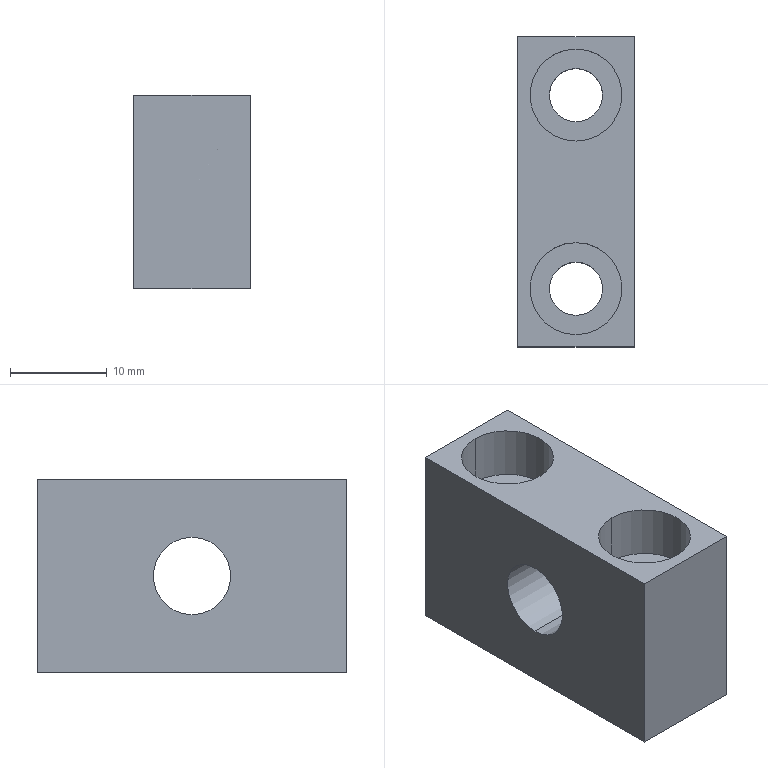Part | STEP file | TNSN20-Y20-F22-Part-13 | 1 solid | 18 faces | box 12 x 32 x 20 mm | volume 5608 mm3 | cylinder 10 | plane 8 | commonest cylinder face diameters 5.5 x4 9.5 x4 8 x2
STEP:
#1=CARTESIAN_POINT('',(14045.745,13720.046,23.));
#2=VERTEX_POINT('',#1);
#3=CARTESIAN_POINT('',(14045.745,13720.046,15.));
#4=VERTEX_POINT('',#3);
#5=CARTESIAN_POINT('',(14045.745,13720.046,19.));
#6=DIRECTION('',(1.,0.,0.));
#7=DIRECTION('',(0.,1.,0.));
#8=AXIS2_PLACEMENT_3D('',#5,#6,#7);
#9=CIRCLE('',#8,4.);
#10=EDGE_CURVE('',#2,#4,#9,.T.);
#11=ORIENTED_EDGE('',*,*,#10,.T.);
#12=CARTESIAN_POINT('',(14033.745,13720.046,15.));
#13=VERTEX_POINT('',#12);
#14=CARTESIAN_POINT('',(14045.745,13720.046,15.));
#15=DIRECTION('',(-1.,0.,0.));
#16=VECTOR('',#15,1000.);
#17=LINE('',#14,#16);
#18=EDGE_CURVE('',#4,#13,#17,.T.);
#19=ORIENTED_EDGE('',*,*,#18,.T.);
#20=CARTESIAN_POINT('',(14033.745,13720.046,23.));
#21=VERTEX_POINT('',#20);
#22=CARTESIAN_POINT('',(14033.745,13720.046,19.));
#23=DIRECTION('',(1.,0.,0.));
#24=DIRECTION('',(0.,1.,0.));
#25=AXIS2_PLACEMENT_3D('',#22,#23,#24);
#26=CIRCLE('',#25,4.);
#27=EDGE_CURVE('',#21,#13,#26,.T.);
#28=ORIENTED_EDGE('',*,*,#27,.F.);
#29=CARTESIAN_POINT('',(14045.745,13720.046,23.));
#30=DIRECTION('',(-1.,0.,0.));
#31=VECTOR('',#30,1000.);
#32=LINE('',#29,#31);
#33=EDGE_CURVE('',#2,#21,#32,.T.);
#34=ORIENTED_EDGE('',*,*,#33,.F.);
#35=EDGE_LOOP('',(#11,#19,#28,#34));
#36=FACE_OUTER_BOUND('',#35,.T.);
#37=CARTESIAN_POINT('',(14045.745,13720.046,19.));
#38=DIRECTION('',(-1.,0.,0.));
#39=DIRECTION('',(0.,0.,1.));
#40=AXIS2_PLACEMENT_3D('',#37,#38,#39);
#41=CYLINDRICAL_SURFACE('',#40,4.);
#42=ADVANCED_FACE('',(#36),#41,.F.);
#43=CARTESIAN_POINT('',(14039.745,13714.796,23.5));
#44=VERTEX_POINT('',#43);
#45=CARTESIAN_POINT('',(14039.745,13705.296,23.5));
#46=VERTEX_POINT('',#45);
#47=CARTESIAN_POINT('',(14039.745,13710.046,23.5));
#48=DIRECTION('',(0.,0.,1.));
#49=DIRECTION('',(1.,0.,0.));
#50=AXIS2_PLACEMENT_3D('',#47,#48,#49);
#51=CIRCLE('',#50,4.75);
#52=EDGE_CURVE('',#44,#46,#51,.T.);
#53=ORIENTED_EDGE('',*,*,#52,.F.);
#54=CARTESIAN_POINT('',(14039.745,13714.796,29.));
#55=VERTEX_POINT('',#54);
#56=CARTESIAN_POINT('',(14039.745,13714.796,26.25));
#57=DIRECTION('',(0.,0.,1.));
#58=VECTOR('',#57,1000.);
#59=LINE('',#56,#58);
#60=EDGE_CURVE('',#44,#55,#59,.T.);
#61=ORIENTED_EDGE('',*,*,#60,.T.);
#62=CARTESIAN_POINT('',(14039.745,13705.296,29.));
#63=VERTEX_POINT('',#62);
#64=CARTESIAN_POINT('',(14039.745,13710.046,29.));
#65=DIRECTION('',(0.,0.,1.));
#66=DIRECTION('',(1.,0.,0.));
#67=AXIS2_PLACEMENT_3D('',#64,#65,#66);
#68=CIRCLE('',#67,4.75);
#69=EDGE_CURVE('',#55,#63,#68,.T.);
#70=ORIENTED_EDGE('',*,*,#69,.T.);
#71=CARTESIAN_POINT('',(14039.745,13705.296,26.25));
#72=DIRECTION('',(0.,0.,1.));
#73=VECTOR('',#72,1000.);
#74=LINE('',#71,#73);
#75=EDGE_CURVE('',#46,#63,#74,.T.);
#76=ORIENTED_EDGE('',*,*,#75,.F.);
#77=EDGE_LOOP('',(#53,#61,#70,#76));
#78=FACE_OUTER_BOUND('',#77,.T.);
#79=CARTESIAN_POINT('',(14039.745,13710.046,26.25));
#80=DIRECTION('',(0.,0.,1.));
#81=DIRECTION('',(0.,-1.,0.));
#82=AXIS2_PLACEMENT_3D('',#79,#80,#81);
#83=CYLINDRICAL_SURFACE('',#82,4.75);
#84=ADVANCED_FACE('',(#78),#83,.F.);
#85=CARTESIAN_POINT('',(14039.745,13734.796,23.5));
#86=VERTEX_POINT('',#85);
#87=CARTESIAN_POINT('',(14039.745,13725.296,23.5));
#88=VERTEX_POINT('',#87);
#89=CARTESIAN_POINT('',(14039.745,13730.046,23.5));
#90=DIRECTION('',(0.,0.,1.));
#91=DIRECTION('',(1.,0.,0.));
#92=AXIS2_PLACEMENT_3D('',#89,#90,#91);
#93=CIRCLE('',#92,4.75);
#94=EDGE_CURVE('',#86,#88,#93,.T.);
#95=ORIENTED_EDGE('',*,*,#94,.F.);
#96=CARTESIAN_POINT('',(14039.745,13734.796,29.));
#97=VERTEX_POINT('',#96);
#98=CARTESIAN_POINT('',(14039.745,13734.796,26.25));
#99=DIRECTION('',(0.,0.,1.));
#100=VECTOR('',#99,1000.);
#101=LINE('',#98,#100);
#102=EDGE_CURVE('',#86,#97,#101,.T.);
#103=ORIENTED_EDGE('',*,*,#102,.T.);
#104=CARTESIAN_POINT('',(14039.745,13725.296,29.));
#105=VERTEX_POINT('',#104);
#106=CARTESIAN_POINT('',(14039.745,13730.046,29.));
#107=DIRECTION('',(0.,0.,1.));
#108=DIRECTION('',(1.,0.,0.));
#109=AXIS2_PLACEMENT_3D('',#106,#107,#108);
#110=CIRCLE('',#109,4.75);
#111=EDGE_CURVE('',#97,#105,#110,.T.);
#112=ORIENTED_EDGE('',*,*,#111,.T.);
#113=CARTESIAN_POINT('',(14039.745,13725.296,26.25));
#114=DIRECTION('',(0.,0.,1.));
#115=VECTOR('',#114,1000.);
#116=LINE('',#113,#115);
#117=EDGE_CURVE('',#88,#105,#116,.T.);
#118=ORIENTED_EDGE('',*,*,#117,.F.);
#119=EDGE_LOOP('',(#95,#103,#112,#118));
#120=FACE_OUTER_BOUND('',#119,.T.);
#121=CARTESIAN_POINT('',(14039.745,13730.046,26.25));
#122=DIRECTION('',(0.,0.,1.));
#123=DIRECTION('',(0.,-1.,0.));
#124=AXIS2_PLACEMENT_3D('',#121,#122,#123);
#125=CYLINDRICAL_SURFACE('',#124,4.75);
#126=ADVANCED_FACE('',(#120),#125,.F.);
#127=CARTESIAN_POINT('',(14039.745,13707.296,23.5));
#128=VERTEX_POINT('',#127);
#129=CARTESIAN_POINT('',(14039.745,13712.796,23.5));
#130=VERTEX_POINT('',#129);
#131=CARTESIAN_POINT('',(14039.745,13710.046,23.5));
#132=DIRECTION('',(0.,0.,1.));
#133=DIRECTION('',(0.,-1.,0.));
#134=AXIS2_PLACEMENT_3D('',#131,#132,#133);
#135=CIRCLE('',#134,2.75);
#136=EDGE_CURVE('',#128,#130,#135,.T.);
#137=ORIENTED_EDGE('',*,*,#136,.T.);
#138=CARTESIAN_POINT('',(14039.745,13712.796,9.));
#139=VERTEX_POINT('',#138);
#140=CARTESIAN_POINT('',(14039.745,13712.796,16.25));
#141=DIRECTION('',(0.,0.,-1.));
#142=VECTOR('',#141,1000.);
#143=LINE('',#140,#142);
#144=EDGE_CURVE('',#130,#139,#143,.T.);
#145=ORIENTED_EDGE('',*,*,#144,.T.);
#146=CARTESIAN_POINT('',(14039.745,13707.296,9.));
#147=VERTEX_POINT('',#146);
#148=CARTESIAN_POINT('',(14039.745,13710.046,9.));
#149=DIRECTION('',(0.,0.,-1.));
#150=DIRECTION('',(0.,1.,0.));
#151=AXIS2_PLACEMENT_3D('',#148,#149,#150);
#152=CIRCLE('',#151,2.75);
#153=EDGE_CURVE('',#139,#147,#152,.T.);
#154=ORIENTED_EDGE('',*,*,#153,.T.);
#155=CARTESIAN_POINT('',(14039.745,13707.296,16.25));
#156=DIRECTION('',(0.,0.,-1.));
#157=VECTOR('',#156,1000.);
#158=LINE('',#155,#157);
#159=EDGE_CURVE('',#128,#147,#158,.T.);
#160=ORIENTED_EDGE('',*,*,#159,.F.);
#161=EDGE_LOOP('',(#137,#145,#154,#160));
#162=FACE_OUTER_BOUND('',#161,.T.);
#163=CARTESIAN_POINT('',(14039.745,13710.046,16.25));
#164=DIRECTION('',(0.,0.,-1.));
#165=DIRECTION('',(0.,-1.,0.));
#166=AXIS2_PLACEMENT_3D('',#163,#164,#165);
#167=CYLINDRICAL_SURFACE('',#166,2.75);
#168=ADVANCED_FACE('',(#162),#167,.F.);
#169=CARTESIAN_POINT('',(14039.745,13727.296,23.5));
#170=VERTEX_POINT('',#169);
#171=CARTESIAN_POINT('',(14039.745,13732.796,23.5));
#172=VERTEX_POINT('',#171);
#173=CARTESIAN_POINT('',(14039.745,13730.046,23.5));
#174=DIRECTION('',(0.,0.,1.));
#175=DIRECTION('',(0.,-1.,0.));
#176=AXIS2_PLACEMENT_3D('',#173,#174,#175);
#177=CIRCLE('',#176,2.75);
#178=EDGE_CURVE('',#170,#172,#177,.T.);
#179=ORIENTED_EDGE('',*,*,#178,.T.);
#180=CARTESIAN_POINT('',(14039.745,13732.796,9.));
#181=VERTEX_POINT('',#180);
#182=CARTESIAN_POINT('',(14039.745,13732.796,16.25));
#183=DIRECTION('',(0.,0.,-1.));
#184=VECTOR('',#183,1000.);
#185=LINE('',#182,#184);
#186=EDGE_CURVE('',#172,#181,#185,.T.);
#187=ORIENTED_EDGE('',*,*,#186,.T.);
#188=CARTESIAN_POINT('',(14039.745,13727.296,9.));
#189=VERTEX_POINT('',#188);
#190=CARTESIAN_POINT('',(14039.745,13730.046,9.));
#191=DIRECTION('',(0.,0.,-1.));
#192=DIRECTION('',(0.,1.,0.));
#193=AXIS2_PLACEMENT_3D('',#190,#191,#192);
#194=CIRCLE('',#193,2.75);
#195=EDGE_CURVE('',#181,#189,#194,.T.);
#196=ORIENTED_EDGE('',*,*,#195,.T.);
#197=CARTESIAN_POINT('',(14039.745,13727.296,16.25));
#198=DIRECTION('',(0.,0.,-1.));
#199=VECTOR('',#198,1000.);
#200=LINE('',#197,#199);
#201=EDGE_CURVE('',#170,#189,#200,.T.);
#202=ORIENTED_EDGE('',*,*,#201,.F.);
#203=EDGE_LOOP('',(#179,#187,#196,#202));
#204=FACE_OUTER_BOUND('',#203,.T.);
#205=CARTESIAN_POINT('',(14039.745,13730.046,16.25));
#206=DIRECTION('',(0.,0.,-1.));
#207=DIRECTION('',(0.,-1.,0.));
#208=AXIS2_PLACEMENT_3D('',#205,#206,#207);
#209=CYLINDRICAL_SURFACE('',#208,2.75);
#210=ADVANCED_FACE('',(#204),#209,.F.);
#211=CARTESIAN_POINT('',(14045.745,13736.046,29.));
#212=VERTEX_POINT('',#211);
#213=CARTESIAN_POINT('',(14033.745,13736.046,29.));
#214=VERTEX_POINT('',#213);
#215=CARTESIAN_POINT('',(14045.745,13736.046,29.));
#216=DIRECTION('',(-1.,0.,0.));
#217=VECTOR('',#216,1000.);
#218=LINE('',#215,#217);
#219=EDGE_CURVE('',#212,#214,#218,.T.);
#220=ORIENTED_EDGE('',*,*,#219,.T.);
#221=CARTESIAN_POINT('',(14033.745,13704.046,29.));
#222=VERTEX_POINT('',#221);
#223=CARTESIAN_POINT('',(14033.745,13704.046,29.));
#224=DIRECTION('',(0.,1.,0.));
#225=VECTOR('',#224,1000.);
#226=LINE('',#223,#225);
#227=EDGE_CURVE('',#222,#214,#226,.T.);
#228=ORIENTED_EDGE('',*,*,#227,.F.);
#229=CARTESIAN_POINT('',(14045.745,13704.046,29.));
#230=VERTEX_POINT('',#229);
#231=CARTESIAN_POINT('',(14045.745,13704.046,29.));
#232=DIRECTION('',(-1.,0.,0.));
#233=VECTOR('',#232,1000.);
#234=LINE('',#231,#233);
#235=EDGE_CURVE('',#230,#222,#234,.T.);
#236=ORIENTED_EDGE('',*,*,#235,.F.);
#237=CARTESIAN_POINT('',(14045.745,13704.046,29.));
#238=DIRECTION('',(0.,1.,0.));
#239=VECTOR('',#238,1000.);
#240=LINE('',#237,#239);
#241=EDGE_CURVE('',#230,#212,#240,.T.);
#242=ORIENTED_EDGE('',*,*,#241,.T.);
#243=EDGE_LOOP('',(#220,#228,#236,#242));
#244=FACE_OUTER_BOUND('',#243,.T.);
#245=CARTESIAN_POINT('',(14039.745,13710.046,29.));
#246=DIRECTION('',(0.,0.,1.));
#247=DIRECTION('',(1.,0.,0.));
#248=AXIS2_PLACEMENT_3D('',#245,#246,#247);
#249=CIRCLE('',#248,4.75);
#250=EDGE_CURVE('',#63,#55,#249,.T.);
#251=ORIENTED_EDGE('',*,*,#250,.F.);
#252=ORIENTED_EDGE('',*,*,#69,.F.);
#253=EDGE_LOOP('',(#251,#252));
#254=FACE_BOUND('',#253,.T.);
#255=CARTESIAN_POINT('',(14039.745,13730.046,29.));
#256=DIRECTION('',(0.,0.,1.));
#257=DIRECTION('',(1.,0.,0.));
#258=AXIS2_PLACEMENT_3D('',#255,#256,#257);
#259=CIRCLE('',#258,4.75);
#260=EDGE_CURVE('',#105,#97,#259,.T.);
#261=ORIENTED_EDGE('',*,*,#260,.F.);
#262=ORIENTED_EDGE('',*,*,#111,.F.);
#263=EDGE_LOOP('',(#261,#262));
#264=FACE_BOUND('',#263,.T.);
#265=CARTESIAN_POINT('',(14008.285,13690.337,29.));
#266=DIRECTION('',(0.,0.,-1.));
#267=DIRECTION('',(0.,1.,0.));
#268=AXIS2_PLACEMENT_3D('',#265,#266,#267);
#269=PLANE('',#268);
#270=ADVANCED_FACE('',(#244,#254,#264),#269,.F.);
#271=CARTESIAN_POINT('',(14033.745,13736.046,9.));
#272=VERTEX_POINT('',#271);
#273=CARTESIAN_POINT('',(14033.745,13736.046,29.));
#274=DIRECTION('',(0.,0.,-1.));
#275=VECTOR('',#274,1000.);
#276=LINE('',#273,#275);
#277=EDGE_CURVE('',#214,#272,#276,.T.);
#278=ORIENTED_EDGE('',*,*,#277,.T.);
#279=CARTESIAN_POINT('',(14033.745,13704.046,9.));
#280=VERTEX_POINT('',#279);
#281=CARTESIAN_POINT('',(14033.745,13704.046,9.));
#282=DIRECTION('',(0.,1.,0.));
#283=VECTOR('',#282,1000.);
#284=LINE('',#281,#283);
#285=EDGE_CURVE('',#280,#272,#284,.T.);
#286=ORIENTED_EDGE('',*,*,#285,.F.);
#287=CARTESIAN_POINT('',(14033.745,13704.046,29.));
#288=DIRECTION('',(0.,0.,-1.));
#289=VECTOR('',#288,1000.);
#290=LINE('',#287,#289);
#291=EDGE_CURVE('',#222,#280,#290,.T.);
#292=ORIENTED_EDGE('',*,*,#291,.F.);
#293=ORIENTED_EDGE('',*,*,#227,.T.);
#294=EDGE_LOOP('',(#278,#286,#292,#293));
#295=FACE_OUTER_BOUND('',#294,.T.);
#296=ORIENTED_EDGE('',*,*,#27,.T.);
#297=CARTESIAN_POINT('',(14033.745,13720.046,19.));
#298=DIRECTION('',(1.,0.,0.));
#299=DIRECTION('',(0.,1.,0.));
#300=AXIS2_PLACEMENT_3D('',#297,#298,#299);
#301=CIRCLE('',#300,4.);
#302=EDGE_CURVE('',#13,#21,#301,.T.);
#303=ORIENTED_EDGE('',*,*,#302,.T.);
#304=EDGE_LOOP('',(#296,#303));
#305=FACE_BOUND('',#304,.T.);
#306=CARTESIAN_POINT('',(14033.745,13691.744,-9.302));
#307=DIRECTION('',(1.,0.,0.));
#308=DIRECTION('',(0.,1.,0.));
#309=AXIS2_PLACEMENT_3D('',#306,#307,#308);
#310=PLANE('',#309);
#311=ADVANCED_FACE('',(#295,#305),#310,.F.);
#312=CARTESIAN_POINT('',(14045.745,13736.046,9.));
#313=VERTEX_POINT('',#312);
#314=CARTESIAN_POINT('',(14033.745,13736.046,9.));
#315=DIRECTION('',(1.,0.,0.));
#316=VECTOR('',#315,1000.);
#317=LINE('',#314,#316);
#318=EDGE_CURVE('',#272,#313,#317,.T.);
#319=ORIENTED_EDGE('',*,*,#318,.T.);
#320=CARTESIAN_POINT('',(14045.745,13704.046,9.));
#321=VERTEX_POINT('',#320);
#322=CARTESIAN_POINT('',(14045.745,13704.046,9.));
#323=DIRECTION('',(0.,1.,0.));
#324=VECTOR('',#323,1000.);
#325=LINE('',#322,#324);
#326=EDGE_CURVE('',#321,#313,#325,.T.);
#327=ORIENTED_EDGE('',*,*,#326,.F.);
#328=CARTESIAN_POINT('',(14033.745,13704.046,9.));
#329=DIRECTION('',(1.,0.,0.));
#330=VECTOR('',#329,1000.);
#331=LINE('',#328,#330);
#332=EDGE_CURVE('',#280,#321,#331,.T.);
#333=ORIENTED_EDGE('',*,*,#332,.F.);
#334=ORIENTED_EDGE('',*,*,#285,.T.);
#335=EDGE_LOOP('',(#319,#327,#333,#334));
#336=FACE_OUTER_BOUND('',#335,.T.);
#337=CARTESIAN_POINT('',(14039.745,13710.046,9.));
#338=DIRECTION('',(0.,0.,-1.));
#339=DIRECTION('',(0.,1.,0.));
#340=AXIS2_PLACEMENT_3D('',#337,#338,#339);
#341=CIRCLE('',#340,2.75);
#342=EDGE_CURVE('',#147,#139,#341,.T.);
#343=ORIENTED_EDGE('',*,*,#342,.F.);
#344=ORIENTED_EDGE('',*,*,#153,.F.);
#345=EDGE_LOOP('',(#343,#344));
#346=FACE_BOUND('',#345,.T.);
#347=CARTESIAN_POINT('',(14039.745,13730.046,9.));
#348=DIRECTION('',(0.,0.,-1.));
#349=DIRECTION('',(0.,1.,0.));
#350=AXIS2_PLACEMENT_3D('',#347,#348,#349);
#351=CIRCLE('',#350,2.75);
#352=EDGE_CURVE('',#189,#181,#351,.T.);
#353=ORIENTED_EDGE('',*,*,#352,.F.);
#354=ORIENTED_EDGE('',*,*,#195,.F.);
#355=EDGE_LOOP('',(#353,#354));
#356=FACE_BOUND('',#355,.T.);
#357=CARTESIAN_POINT('',(14014.113,13745.678,9.));
#358=DIRECTION('',(0.,0.,1.));
#359=DIRECTION('',(0.,-1.,0.));
#360=AXIS2_PLACEMENT_3D('',#357,#358,#359);
#361=PLANE('',#360);
#362=ADVANCED_FACE('',(#336,#346,#356),#361,.F.);
#363=CARTESIAN_POINT('',(14045.745,13736.046,9.));
#364=DIRECTION('',(0.,0.,1.));
#365=VECTOR('',#364,1000.);
#366=LINE('',#363,#365);
#367=EDGE_CURVE('',#313,#212,#366,.T.);
#368=ORIENTED_EDGE('',*,*,#367,.T.);
#369=ORIENTED_EDGE('',*,*,#241,.F.);
#370=CARTESIAN_POINT('',(14045.745,13704.046,9.));
#371=DIRECTION('',(0.,0.,1.));
#372=VECTOR('',#371,1000.);
#373=LINE('',#370,#372);
#374=EDGE_CURVE('',#321,#230,#373,.T.);
#375=ORIENTED_EDGE('',*,*,#374,.F.);
#376=ORIENTED_EDGE('',*,*,#326,.T.);
#377=EDGE_LOOP('',(#368,#369,#375,#376));
#378=FACE_OUTER_BOUND('',#377,.T.);
#379=ORIENTED_EDGE('',*,*,#10,.F.);
#380=CARTESIAN_POINT('',(14045.745,13720.046,19.));
#381=DIRECTION('',(1.,0.,0.));
#382=DIRECTION('',(0.,1.,0.));
#383=AXIS2_PLACEMENT_3D('',#380,#381,#382);
#384=CIRCLE('',#383,4.);
#385=EDGE_CURVE('',#4,#2,#384,.T.);
#386=ORIENTED_EDGE('',*,*,#385,.F.);
#387=EDGE_LOOP('',(#379,#386));
#388=FACE_BOUND('',#387,.T.);
#389=CARTESIAN_POINT('',(14045.745,13748.348,-9.302));
#390=DIRECTION('',(-1.,0.,0.));
#391=DIRECTION('',(0.,-1.,0.));
#392=AXIS2_PLACEMENT_3D('',#389,#390,#391);
#393=PLANE('',#392);
#394=ADVANCED_FACE('',(#378,#388),#393,.F.);
#395=ORIENTED_EDGE('',*,*,#235,.T.);
#396=ORIENTED_EDGE('',*,*,#291,.T.);
#397=ORIENTED_EDGE('',*,*,#332,.T.);
#398=ORIENTED_EDGE('',*,*,#374,.T.);
#399=EDGE_LOOP('',(#395,#396,#397,#398));
#400=FACE_OUTER_BOUND('',#399,.T.);
#401=CARTESIAN_POINT('',(14022.252,13704.046,1.507));
#402=DIRECTION('',(0.,-1.,0.));
#403=DIRECTION('',(1.,0.,0.));
#404=AXIS2_PLACEMENT_3D('',#401,#402,#403);
#405=PLANE('',#404);
#406=ADVANCED_FACE('',(#400),#405,.T.);
#407=ORIENTED_EDGE('',*,*,#219,.F.);
#408=ORIENTED_EDGE('',*,*,#367,.F.);
#409=ORIENTED_EDGE('',*,*,#318,.F.);
#410=ORIENTED_EDGE('',*,*,#277,.F.);
#411=EDGE_LOOP('',(#407,#408,#409,#410));
#412=FACE_OUTER_BOUND('',#411,.T.);
#413=CARTESIAN_POINT('',(14022.252,13736.046,1.507));
#414=DIRECTION('',(0.,-1.,0.));
#415=DIRECTION('',(1.,0.,0.));
#416=AXIS2_PLACEMENT_3D('',#413,#414,#415);
#417=PLANE('',#416);
#418=ADVANCED_FACE('',(#412),#417,.F.);
#419=CARTESIAN_POINT('',(14039.745,13730.046,23.5));
#420=DIRECTION('',(0.,0.,1.));
#421=DIRECTION('',(1.,0.,0.));
#422=AXIS2_PLACEMENT_3D('',#419,#420,#421);
#423=CIRCLE('',#422,4.75);
#424=EDGE_CURVE('',#88,#86,#423,.T.);
#425=ORIENTED_EDGE('',*,*,#424,.T.);
#426=ORIENTED_EDGE('',*,*,#94,.T.);
#427=EDGE_LOOP('',(#425,#426));
#428=FACE_OUTER_BOUND('',#427,.T.);
#429=ORIENTED_EDGE('',*,*,#178,.F.);
#430=CARTESIAN_POINT('',(14039.745,13730.046,23.5));
#431=DIRECTION('',(0.,0.,1.));
#432=DIRECTION('',(0.,-1.,0.));
#433=AXIS2_PLACEMENT_3D('',#430,#431,#432);
#434=CIRCLE('',#433,2.75);
#435=EDGE_CURVE('',#172,#170,#434,.T.);
#436=ORIENTED_EDGE('',*,*,#435,.F.);
#437=EDGE_LOOP('',(#429,#436));
#438=FACE_BOUND('',#437,.T.);
#439=CARTESIAN_POINT('',(14021.045,13746.378,23.5));
#440=DIRECTION('',(0.,0.,1.));
#441=DIRECTION('',(0.,-1.,0.));
#442=AXIS2_PLACEMENT_3D('',#439,#440,#441);
#443=PLANE('',#442);
#444=ADVANCED_FACE('',(#428,#438),#443,.T.);
#445=CARTESIAN_POINT('',(14039.745,13710.046,23.5));
#446=DIRECTION('',(0.,0.,1.));
#447=DIRECTION('',(1.,0.,0.));
#448=AXIS2_PLACEMENT_3D('',#445,#446,#447);
#449=CIRCLE('',#448,4.75);
#450=EDGE_CURVE('',#46,#44,#449,.T.);
#451=ORIENTED_EDGE('',*,*,#450,.T.);
#452=ORIENTED_EDGE('',*,*,#52,.T.);
#453=EDGE_LOOP('',(#451,#452));
#454=FACE_OUTER_BOUND('',#453,.T.);
#455=ORIENTED_EDGE('',*,*,#136,.F.);
#456=CARTESIAN_POINT('',(14039.745,13710.046,23.5));
#457=DIRECTION('',(0.,0.,1.));
#458=DIRECTION('',(0.,-1.,0.));
#459=AXIS2_PLACEMENT_3D('',#456,#457,#458);
#460=CIRCLE('',#459,2.75);
#461=EDGE_CURVE('',#130,#128,#460,.T.);
#462=ORIENTED_EDGE('',*,*,#461,.F.);
#463=EDGE_LOOP('',(#455,#462));
#464=FACE_BOUND('',#463,.T.);
#465=CARTESIAN_POINT('',(14021.045,13726.378,23.5));
#466=DIRECTION('',(0.,0.,1.));
#467=DIRECTION('',(0.,-1.,0.));
#468=AXIS2_PLACEMENT_3D('',#465,#466,#467);
#469=PLANE('',#468);
#470=ADVANCED_FACE('',(#454,#464),#469,.T.);
#471=ORIENTED_EDGE('',*,*,#186,.F.);
#472=ORIENTED_EDGE('',*,*,#435,.T.);
#473=ORIENTED_EDGE('',*,*,#201,.T.);
#474=ORIENTED_EDGE('',*,*,#352,.T.);
#475=EDGE_LOOP('',(#471,#472,#473,#474));
#476=FACE_OUTER_BOUND('',#475,.T.);
#477=CARTESIAN_POINT('',(14039.745,13730.046,16.25));
#478=DIRECTION('',(0.,0.,-1.));
#479=DIRECTION('',(0.,-1.,0.));
#480=AXIS2_PLACEMENT_3D('',#477,#478,#479);
#481=CYLINDRICAL_SURFACE('',#480,2.75);
#482=ADVANCED_FACE('',(#476),#481,.F.);
#483=ORIENTED_EDGE('',*,*,#144,.F.);
#484=ORIENTED_EDGE('',*,*,#461,.T.);
#485=ORIENTED_EDGE('',*,*,#159,.T.);
#486=ORIENTED_EDGE('',*,*,#342,.T.);
#487=EDGE_LOOP('',(#483,#484,#485,#486));
#488=FACE_OUTER_BOUND('',#487,.T.);
#489=CARTESIAN_POINT('',(14039.745,13710.046,16.25));
#490=DIRECTION('',(0.,0.,-1.));
#491=DIRECTION('',(0.,-1.,0.));
#492=AXIS2_PLACEMENT_3D('',#489,#490,#491);
#493=CYLINDRICAL_SURFACE('',#492,2.75);
#494=ADVANCED_FACE('',(#488),#493,.F.);
#495=ORIENTED_EDGE('',*,*,#102,.F.);
#496=ORIENTED_EDGE('',*,*,#424,.F.);
#497=ORIENTED_EDGE('',*,*,#117,.T.);
#498=ORIENTED_EDGE('',*,*,#260,.T.);
#499=EDGE_LOOP('',(#495,#496,#497,#498));
#500=FACE_OUTER_BOUND('',#499,.T.);
#501=CARTESIAN_POINT('',(14039.745,13730.046,26.25));
#502=DIRECTION('',(0.,0.,1.));
#503=DIRECTION('',(0.,-1.,0.));
#504=AXIS2_PLACEMENT_3D('',#501,#502,#503);
#505=CYLINDRICAL_SURFACE('',#504,4.75);
#506=ADVANCED_FACE('',(#500),#505,.F.);
#507=ORIENTED_EDGE('',*,*,#60,.F.);
#508=ORIENTED_EDGE('',*,*,#450,.F.);
#509=ORIENTED_EDGE('',*,*,#75,.T.);
#510=ORIENTED_EDGE('',*,*,#250,.T.);
#511=EDGE_LOOP('',(#507,#508,#509,#510));
#512=FACE_OUTER_BOUND('',#511,.T.);
#513=CARTESIAN_POINT('',(14039.745,13710.046,26.25));
#514=DIRECTION('',(0.,0.,1.));
#515=DIRECTION('',(0.,-1.,0.));
#516=AXIS2_PLACEMENT_3D('',#513,#514,#515);
#517=CYLINDRICAL_SURFACE('',#516,4.75);
#518=ADVANCED_FACE('',(#512),#517,.F.);
#519=ORIENTED_EDGE('',*,*,#18,.F.);
#520=ORIENTED_EDGE('',*,*,#385,.T.);
#521=ORIENTED_EDGE('',*,*,#33,.T.);
#522=ORIENTED_EDGE('',*,*,#302,.F.);
#523=EDGE_LOOP('',(#519,#520,#521,#522));
#524=FACE_OUTER_BOUND('',#523,.T.);
#525=CARTESIAN_POINT('',(14045.745,13720.046,19.));
#526=DIRECTION('',(-1.,0.,0.));
#527=DIRECTION('',(0.,0.,1.));
#528=AXIS2_PLACEMENT_3D('',#525,#526,#527);
#529=CYLINDRICAL_SURFACE('',#528,4.);
#530=ADVANCED_FACE('',(#524),#529,.F.);
#531=CLOSED_SHELL('',(#42,#84,#126,#168,#210,#270,#311,#362,#394,#406,#418,#444,#470,#482,#494,#506,#518,#530));
#532=MANIFOLD_SOLID_BREP('',#531);
#533=CARTESIAN_POINT('',(0.,0.,0.));
#534=DIRECTION('',(0.,0.,1.));
#535=DIRECTION('',(1.,0.,0.));
#536=AXIS2_PLACEMENT_3D('',#533,#534,#535);
#537=(LENGTH_UNIT()NAMED_UNIT(*)SI_UNIT(.MILLI.,.METRE.));
#538=UNCERTAINTY_MEASURE_WITH_UNIT(LENGTH_MEASURE(0.00001),#537,'','');
#539=(NAMED_UNIT(*)PLANE_ANGLE_UNIT()SI_UNIT($,.RADIAN.));
#540=(NAMED_UNIT(*)SI_UNIT($,.STERADIAN.)SOLID_ANGLE_UNIT());
#541=(GEOMETRIC_REPRESENTATION_CONTEXT(3)GLOBAL_UNCERTAINTY_ASSIGNED_CONTEXT((#538))GLOBAL_UNIT_ASSIGNED_CONTEXT((#537,#539,#540))REPRESENTATION_CONTEXT('',''));
#542=ADVANCED_BREP_SHAPE_REPRESENTATION('',(#532,#536),#541);